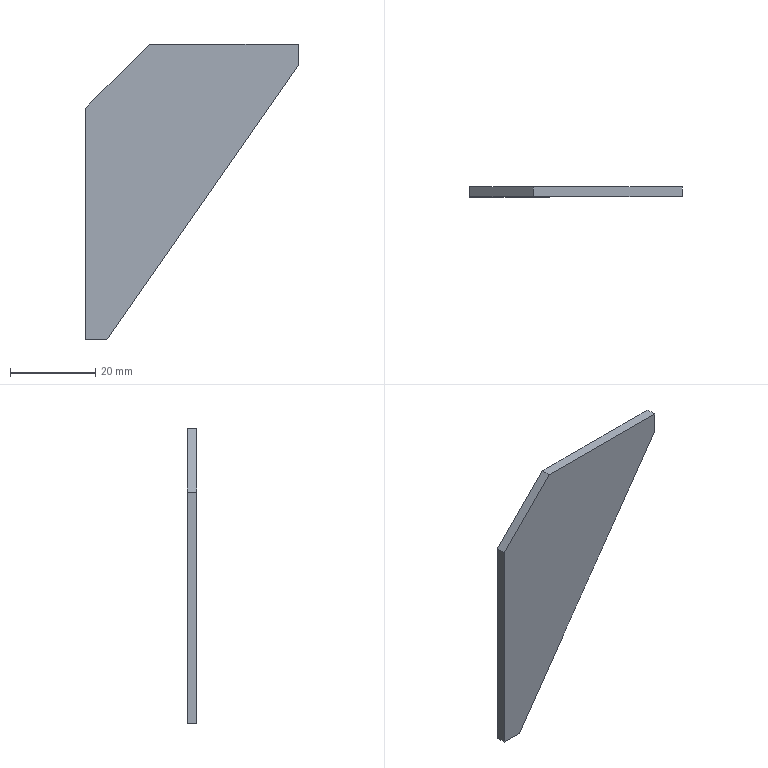Part | SolidWorks | features FlatPattern 1, SMBaseFlange 1, SheetMetal 1 | 1 solid | 8 faces | box 50 x 2.3 x 69.5 mm | volume 4396 mm3 | plane 8
STEP:
#1=CARTESIAN_POINT('',(5.,0.,0.));
#2=VERTEX_POINT('',#1);
#3=CARTESIAN_POINT('',(0.,0.,0.));
#4=VERTEX_POINT('',#3);
#5=CARTESIAN_POINT('',(5.,0.,0.));
#6=DIRECTION('',(-1.,0.,0.));
#7=VECTOR('',#6,1000.);
#8=LINE('',#5,#7);
#9=EDGE_CURVE('',#2,#4,#8,.T.);
#10=ORIENTED_EDGE('',*,*,#9,.F.);
#11=CARTESIAN_POINT('',(5.,-2.3,0.));
#12=VERTEX_POINT('',#11);
#13=CARTESIAN_POINT('',(5.,-2.3,0.));
#14=DIRECTION('',(0.,1.,0.));
#15=VECTOR('',#14,1000.);
#16=LINE('',#13,#15);
#17=EDGE_CURVE('',#12,#2,#16,.T.);
#18=ORIENTED_EDGE('',*,*,#17,.F.);
#19=CARTESIAN_POINT('',(0.,-2.3,0.));
#20=VERTEX_POINT('',#19);
#21=CARTESIAN_POINT('',(5.,-2.3,0.));
#22=DIRECTION('',(-1.,0.,0.));
#23=VECTOR('',#22,1000.);
#24=LINE('',#21,#23);
#25=EDGE_CURVE('',#12,#20,#24,.T.);
#26=ORIENTED_EDGE('',*,*,#25,.T.);
#27=CARTESIAN_POINT('',(0.,-2.3,0.));
#28=DIRECTION('',(0.,1.,0.));
#29=VECTOR('',#28,1000.);
#30=LINE('',#27,#29);
#31=EDGE_CURVE('',#20,#4,#30,.T.);
#32=ORIENTED_EDGE('',*,*,#31,.T.);
#33=EDGE_LOOP('',(#10,#18,#26,#32));
#34=FACE_OUTER_BOUND('',#33,.T.);
#35=CARTESIAN_POINT('',(5.,-2.3,0.));
#36=DIRECTION('',(0.,0.,-1.));
#37=DIRECTION('',(-1.,0.,0.));
#38=AXIS2_PLACEMENT_3D('',#35,#36,#37);
#39=PLANE('',#38);
#40=ADVANCED_FACE('',(#34),#39,.T.);
#41=CARTESIAN_POINT('',(50.,0.,64.5));
#42=VERTEX_POINT('',#41);
#43=CARTESIAN_POINT('',(50.,0.,64.5));
#44=DIRECTION('',(-0.5722,0.,-0.8201));
#45=VECTOR('',#44,1000.);
#46=LINE('',#43,#45);
#47=EDGE_CURVE('',#42,#2,#46,.T.);
#48=ORIENTED_EDGE('',*,*,#47,.F.);
#49=CARTESIAN_POINT('',(50.,-2.3,64.5));
#50=VERTEX_POINT('',#49);
#51=CARTESIAN_POINT('',(50.,-2.3,64.5));
#52=DIRECTION('',(0.,1.,0.));
#53=VECTOR('',#52,1000.);
#54=LINE('',#51,#53);
#55=EDGE_CURVE('',#50,#42,#54,.T.);
#56=ORIENTED_EDGE('',*,*,#55,.F.);
#57=CARTESIAN_POINT('',(50.,-2.3,64.5));
#58=DIRECTION('',(-0.5722,0.,-0.8201));
#59=VECTOR('',#58,1000.);
#60=LINE('',#57,#59);
#61=EDGE_CURVE('',#50,#12,#60,.T.);
#62=ORIENTED_EDGE('',*,*,#61,.T.);
#63=ORIENTED_EDGE('',*,*,#17,.T.);
#64=EDGE_LOOP('',(#48,#56,#62,#63));
#65=FACE_OUTER_BOUND('',#64,.T.);
#66=CARTESIAN_POINT('',(50.,-2.3,64.5));
#67=DIRECTION('',(0.8201,0.,-0.5722));
#68=DIRECTION('',(-0.5722,0.,-0.8201));
#69=AXIS2_PLACEMENT_3D('',#66,#67,#68);
#70=PLANE('',#69);
#71=ADVANCED_FACE('',(#65),#70,.T.);
#72=CARTESIAN_POINT('',(50.,0.,69.5));
#73=VERTEX_POINT('',#72);
#74=CARTESIAN_POINT('',(50.,0.,69.5));
#75=DIRECTION('',(0.,0.,-1.));
#76=VECTOR('',#75,1000.);
#77=LINE('',#74,#76);
#78=EDGE_CURVE('',#73,#42,#77,.T.);
#79=ORIENTED_EDGE('',*,*,#78,.F.);
#80=CARTESIAN_POINT('',(50.,-2.3,69.5));
#81=VERTEX_POINT('',#80);
#82=CARTESIAN_POINT('',(50.,-2.3,69.5));
#83=DIRECTION('',(0.,1.,0.));
#84=VECTOR('',#83,1000.);
#85=LINE('',#82,#84);
#86=EDGE_CURVE('',#81,#73,#85,.T.);
#87=ORIENTED_EDGE('',*,*,#86,.F.);
#88=CARTESIAN_POINT('',(50.,-2.3,69.5));
#89=DIRECTION('',(0.,0.,-1.));
#90=VECTOR('',#89,1000.);
#91=LINE('',#88,#90);
#92=EDGE_CURVE('',#81,#50,#91,.T.);
#93=ORIENTED_EDGE('',*,*,#92,.T.);
#94=ORIENTED_EDGE('',*,*,#55,.T.);
#95=EDGE_LOOP('',(#79,#87,#93,#94));
#96=FACE_OUTER_BOUND('',#95,.T.);
#97=CARTESIAN_POINT('',(50.,-2.3,69.5));
#98=DIRECTION('',(1.,0.,0.));
#99=DIRECTION('',(0.,0.,-1.));
#100=AXIS2_PLACEMENT_3D('',#97,#98,#99);
#101=PLANE('',#100);
#102=ADVANCED_FACE('',(#96),#101,.T.);
#103=CARTESIAN_POINT('',(15.,0.,69.5));
#104=VERTEX_POINT('',#103);
#105=CARTESIAN_POINT('',(15.,0.,69.5));
#106=DIRECTION('',(1.,0.,0.));
#107=VECTOR('',#106,1000.);
#108=LINE('',#105,#107);
#109=EDGE_CURVE('',#104,#73,#108,.T.);
#110=ORIENTED_EDGE('',*,*,#109,.F.);
#111=CARTESIAN_POINT('',(15.,-2.3,69.5));
#112=VERTEX_POINT('',#111);
#113=CARTESIAN_POINT('',(15.,-2.3,69.5));
#114=DIRECTION('',(0.,1.,0.));
#115=VECTOR('',#114,1000.);
#116=LINE('',#113,#115);
#117=EDGE_CURVE('',#112,#104,#116,.T.);
#118=ORIENTED_EDGE('',*,*,#117,.F.);
#119=CARTESIAN_POINT('',(15.,-2.3,69.5));
#120=DIRECTION('',(1.,0.,0.));
#121=VECTOR('',#120,1000.);
#122=LINE('',#119,#121);
#123=EDGE_CURVE('',#112,#81,#122,.T.);
#124=ORIENTED_EDGE('',*,*,#123,.T.);
#125=ORIENTED_EDGE('',*,*,#86,.T.);
#126=EDGE_LOOP('',(#110,#118,#124,#125));
#127=FACE_OUTER_BOUND('',#126,.T.);
#128=CARTESIAN_POINT('',(15.,-2.3,69.5));
#129=DIRECTION('',(0.,0.,1.));
#130=DIRECTION('',(1.,0.,0.));
#131=AXIS2_PLACEMENT_3D('',#128,#129,#130);
#132=PLANE('',#131);
#133=ADVANCED_FACE('',(#127),#132,.T.);
#134=CARTESIAN_POINT('',(0.,0.,54.5));
#135=VERTEX_POINT('',#134);
#136=CARTESIAN_POINT('',(0.,0.,54.5));
#137=DIRECTION('',(0.7071,0.,0.7071));
#138=VECTOR('',#137,1000.);
#139=LINE('',#136,#138);
#140=EDGE_CURVE('',#135,#104,#139,.T.);
#141=ORIENTED_EDGE('',*,*,#140,.F.);
#142=CARTESIAN_POINT('',(0.,-2.3,54.5));
#143=VERTEX_POINT('',#142);
#144=CARTESIAN_POINT('',(0.,-2.3,54.5));
#145=DIRECTION('',(0.,1.,0.));
#146=VECTOR('',#145,1000.);
#147=LINE('',#144,#146);
#148=EDGE_CURVE('',#143,#135,#147,.T.);
#149=ORIENTED_EDGE('',*,*,#148,.F.);
#150=CARTESIAN_POINT('',(0.,-2.3,54.5));
#151=DIRECTION('',(0.7071,0.,0.7071));
#152=VECTOR('',#151,1000.);
#153=LINE('',#150,#152);
#154=EDGE_CURVE('',#143,#112,#153,.T.);
#155=ORIENTED_EDGE('',*,*,#154,.T.);
#156=ORIENTED_EDGE('',*,*,#117,.T.);
#157=EDGE_LOOP('',(#141,#149,#155,#156));
#158=FACE_OUTER_BOUND('',#157,.T.);
#159=CARTESIAN_POINT('',(0.,-2.3,54.5));
#160=DIRECTION('',(-0.7071,0.,0.7071));
#161=DIRECTION('',(0.7071,0.,0.7071));
#162=AXIS2_PLACEMENT_3D('',#159,#160,#161);
#163=PLANE('',#162);
#164=ADVANCED_FACE('',(#158),#163,.T.);
#165=CARTESIAN_POINT('',(0.,0.,0.));
#166=DIRECTION('',(0.,0.,1.));
#167=VECTOR('',#166,1000.);
#168=LINE('',#165,#167);
#169=EDGE_CURVE('',#4,#135,#168,.T.);
#170=ORIENTED_EDGE('',*,*,#169,.F.);
#171=ORIENTED_EDGE('',*,*,#31,.F.);
#172=CARTESIAN_POINT('',(0.,-2.3,0.));
#173=DIRECTION('',(0.,0.,1.));
#174=VECTOR('',#173,1000.);
#175=LINE('',#172,#174);
#176=EDGE_CURVE('',#20,#143,#175,.T.);
#177=ORIENTED_EDGE('',*,*,#176,.T.);
#178=ORIENTED_EDGE('',*,*,#148,.T.);
#179=EDGE_LOOP('',(#170,#171,#177,#178));
#180=FACE_OUTER_BOUND('',#179,.T.);
#181=CARTESIAN_POINT('',(0.,-2.3,0.));
#182=DIRECTION('',(-1.,0.,0.));
#183=DIRECTION('',(0.,0.,1.));
#184=AXIS2_PLACEMENT_3D('',#181,#182,#183);
#185=PLANE('',#184);
#186=ADVANCED_FACE('',(#180),#185,.T.);
#187=ORIENTED_EDGE('',*,*,#25,.F.);
#188=ORIENTED_EDGE('',*,*,#61,.F.);
#189=ORIENTED_EDGE('',*,*,#92,.F.);
#190=ORIENTED_EDGE('',*,*,#123,.F.);
#191=ORIENTED_EDGE('',*,*,#154,.F.);
#192=ORIENTED_EDGE('',*,*,#176,.F.);
#193=EDGE_LOOP('',(#187,#188,#189,#190,#191,#192));
#194=FACE_OUTER_BOUND('',#193,.T.);
#195=CARTESIAN_POINT('',(0.,-2.3,0.));
#196=DIRECTION('',(0.,1.,0.));
#197=DIRECTION('',(0.,0.,1.));
#198=AXIS2_PLACEMENT_3D('',#195,#196,#197);
#199=PLANE('',#198);
#200=ADVANCED_FACE('',(#194),#199,.F.);
#201=ORIENTED_EDGE('',*,*,#9,.T.);
#202=ORIENTED_EDGE('',*,*,#169,.T.);
#203=ORIENTED_EDGE('',*,*,#140,.T.);
#204=ORIENTED_EDGE('',*,*,#109,.T.);
#205=ORIENTED_EDGE('',*,*,#78,.T.);
#206=ORIENTED_EDGE('',*,*,#47,.T.);
#207=EDGE_LOOP('',(#201,#202,#203,#204,#205,#206));
#208=FACE_OUTER_BOUND('',#207,.T.);
#209=CARTESIAN_POINT('',(0.,0.,0.));
#210=DIRECTION('',(0.,1.,0.));
#211=DIRECTION('',(0.,0.,1.));
#212=AXIS2_PLACEMENT_3D('',#209,#210,#211);
#213=PLANE('',#212);
#214=ADVANCED_FACE('',(#208),#213,.T.);
#215=CLOSED_SHELL('',(#40,#71,#102,#133,#164,#186,#200,#214));
#216=MANIFOLD_SOLID_BREP('',#215);
#217=CARTESIAN_POINT('',(0.,0.,0.));
#218=DIRECTION('',(0.,0.,1.));
#219=DIRECTION('',(1.,0.,0.));
#220=AXIS2_PLACEMENT_3D('',#217,#218,#219);
#221=(LENGTH_UNIT()NAMED_UNIT(*)SI_UNIT(.MILLI.,.METRE.));
#222=UNCERTAINTY_MEASURE_WITH_UNIT(LENGTH_MEASURE(0.00001),#221,'','');
#223=(NAMED_UNIT(*)PLANE_ANGLE_UNIT()SI_UNIT($,.RADIAN.));
#224=(NAMED_UNIT(*)SI_UNIT($,.STERADIAN.)SOLID_ANGLE_UNIT());
#225=(GEOMETRIC_REPRESENTATION_CONTEXT(3)GLOBAL_UNCERTAINTY_ASSIGNED_CONTEXT((#222))GLOBAL_UNIT_ASSIGNED_CONTEXT((#221,#223,#224))REPRESENTATION_CONTEXT('',''));
#226=ADVANCED_BREP_SHAPE_REPRESENTATION('',(#216,#220),#225);